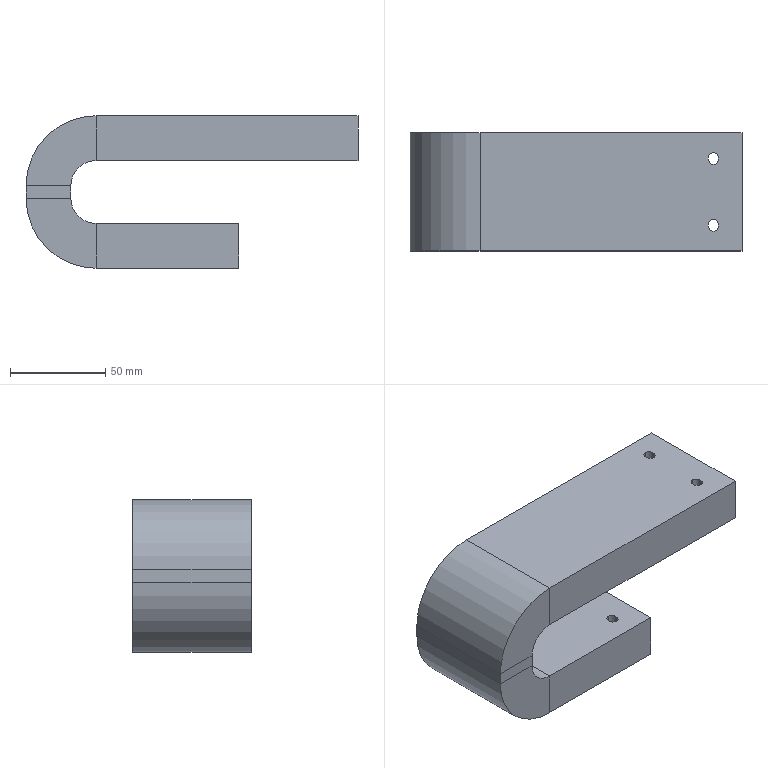Part | SolidWorks | features HoleWzd 2, Sweep 1 | 1 solid | 42 faces | box 174.25 x 62 x 80 mm | volume 431030 mm3 | plane 26 | cylinder 16 | commonest cylinder face diameters 5.2 x12 26.5 x2 73.5 x2
STEP:
#1=CARTESIAN_POINT('',(-15.,-14.4,11.75));
#2=VERTEX_POINT('',#1);
#3=CARTESIAN_POINT('',(-12.4,-17.,11.75));
#4=VERTEX_POINT('',#3);
#5=CARTESIAN_POINT('',(-15.,-17.,11.75));
#6=DIRECTION('',(0.,0.,-1.));
#7=DIRECTION('',(-1.,0.,0.));
#8=AXIS2_PLACEMENT_3D('',#5,#6,#7);
#9=CIRCLE('',#8,2.6);
#10=EDGE_CURVE('',#2,#4,#9,.T.);
#11=ORIENTED_EDGE('',*,*,#10,.F.);
#12=CARTESIAN_POINT('',(-15.,-14.4,-11.75));
#13=VERTEX_POINT('',#12);
#14=CARTESIAN_POINT('',(-15.,-14.4,-11.75));
#15=DIRECTION('',(0.,0.,-1.));
#16=VECTOR('',#15,1000.);
#17=LINE('',#14,#16);
#18=EDGE_CURVE('',#2,#13,#17,.T.);
#19=ORIENTED_EDGE('',*,*,#18,.T.);
#20=CARTESIAN_POINT('',(-12.4,-17.,-11.75));
#21=VERTEX_POINT('',#20);
#22=CARTESIAN_POINT('',(-15.,-17.,-11.75));
#23=DIRECTION('',(0.,0.,-1.));
#24=DIRECTION('',(0.,1.,0.));
#25=AXIS2_PLACEMENT_3D('',#22,#23,#24);
#26=CIRCLE('',#25,2.6);
#27=EDGE_CURVE('',#13,#21,#26,.T.);
#28=ORIENTED_EDGE('',*,*,#27,.T.);
#29=CARTESIAN_POINT('',(-12.4,-17.,23.25));
#30=DIRECTION('',(0.,0.,1.));
#31=VECTOR('',#30,1000.);
#32=LINE('',#29,#31);
#33=EDGE_CURVE('',#21,#4,#32,.T.);
#34=ORIENTED_EDGE('',*,*,#33,.T.);
#35=EDGE_LOOP('',(#11,#19,#28,#34));
#36=FACE_OUTER_BOUND('',#35,.T.);
#37=CARTESIAN_POINT('',(-15.,-17.,-11.75));
#38=DIRECTION('',(0.,0.,-1.));
#39=DIRECTION('',(0.,1.,0.));
#40=AXIS2_PLACEMENT_3D('',#37,#38,#39);
#41=CYLINDRICAL_SURFACE('',#40,2.6);
#42=ADVANCED_FACE('',(#36),#41,.F.);
#43=CARTESIAN_POINT('',(-15.,20.6,11.75));
#44=VERTEX_POINT('',#43);
#45=CARTESIAN_POINT('',(-12.4,18.,11.75));
#46=VERTEX_POINT('',#45);
#47=CARTESIAN_POINT('',(-15.,18.,11.75));
#48=DIRECTION('',(0.,0.,-1.));
#49=DIRECTION('',(-1.,0.,0.));
#50=AXIS2_PLACEMENT_3D('',#47,#48,#49);
#51=CIRCLE('',#50,2.6);
#52=EDGE_CURVE('',#44,#46,#51,.T.);
#53=ORIENTED_EDGE('',*,*,#52,.F.);
#54=CARTESIAN_POINT('',(-15.,20.6,-11.75));
#55=VERTEX_POINT('',#54);
#56=CARTESIAN_POINT('',(-15.,20.6,-11.75));
#57=DIRECTION('',(0.,0.,-1.));
#58=VECTOR('',#57,1000.);
#59=LINE('',#56,#58);
#60=EDGE_CURVE('',#44,#55,#59,.T.);
#61=ORIENTED_EDGE('',*,*,#60,.T.);
#62=CARTESIAN_POINT('',(-12.4,18.,-11.75));
#63=VERTEX_POINT('',#62);
#64=CARTESIAN_POINT('',(-15.,18.,-11.75));
#65=DIRECTION('',(0.,0.,-1.));
#66=DIRECTION('',(0.,1.,0.));
#67=AXIS2_PLACEMENT_3D('',#64,#65,#66);
#68=CIRCLE('',#67,2.6);
#69=EDGE_CURVE('',#55,#63,#68,.T.);
#70=ORIENTED_EDGE('',*,*,#69,.T.);
#71=CARTESIAN_POINT('',(-12.4,18.,23.25));
#72=DIRECTION('',(0.,0.,1.));
#73=VECTOR('',#72,1000.);
#74=LINE('',#71,#73);
#75=EDGE_CURVE('',#63,#46,#74,.T.);
#76=ORIENTED_EDGE('',*,*,#75,.T.);
#77=EDGE_LOOP('',(#53,#61,#70,#76));
#78=FACE_OUTER_BOUND('',#77,.T.);
#79=CARTESIAN_POINT('',(-15.,18.,-11.75));
#80=DIRECTION('',(0.,0.,-1.));
#81=DIRECTION('',(0.,1.,0.));
#82=AXIS2_PLACEMENT_3D('',#79,#80,#81);
#83=CYLINDRICAL_SURFACE('',#82,2.6);
#84=ADVANCED_FACE('',(#78),#83,.F.);
#85=CARTESIAN_POINT('',(47.5,-14.4,68.25));
#86=VERTEX_POINT('',#85);
#87=CARTESIAN_POINT('',(50.1,-17.,68.25));
#88=VERTEX_POINT('',#87);
#89=CARTESIAN_POINT('',(47.5,-17.,68.25));
#90=DIRECTION('',(0.,0.,-1.));
#91=DIRECTION('',(0.,1.,0.));
#92=AXIS2_PLACEMENT_3D('',#89,#90,#91);
#93=CIRCLE('',#92,2.6);
#94=EDGE_CURVE('',#86,#88,#93,.T.);
#95=ORIENTED_EDGE('',*,*,#94,.F.);
#96=CARTESIAN_POINT('',(47.5,-14.4,44.75));
#97=VERTEX_POINT('',#96);
#98=CARTESIAN_POINT('',(47.5,-14.4,44.75));
#99=DIRECTION('',(0.,0.,-1.));
#100=VECTOR('',#99,1000.);
#101=LINE('',#98,#100);
#102=EDGE_CURVE('',#86,#97,#101,.T.);
#103=ORIENTED_EDGE('',*,*,#102,.T.);
#104=CARTESIAN_POINT('',(50.1,-17.,44.75));
#105=VERTEX_POINT('',#104);
#106=CARTESIAN_POINT('',(47.5,-17.,44.75));
#107=DIRECTION('',(0.,0.,-1.));
#108=DIRECTION('',(0.,1.,0.));
#109=AXIS2_PLACEMENT_3D('',#106,#107,#108);
#110=CIRCLE('',#109,2.6);
#111=EDGE_CURVE('',#97,#105,#110,.T.);
#112=ORIENTED_EDGE('',*,*,#111,.T.);
#113=CARTESIAN_POINT('',(50.1,-17.,68.25));
#114=DIRECTION('',(0.,0.,1.));
#115=VECTOR('',#114,1000.);
#116=LINE('',#113,#115);
#117=EDGE_CURVE('',#105,#88,#116,.T.);
#118=ORIENTED_EDGE('',*,*,#117,.T.);
#119=EDGE_LOOP('',(#95,#103,#112,#118));
#120=FACE_OUTER_BOUND('',#119,.T.);
#121=CARTESIAN_POINT('',(47.5,-17.,44.75));
#122=DIRECTION('',(0.,0.,-1.));
#123=DIRECTION('',(0.,1.,0.));
#124=AXIS2_PLACEMENT_3D('',#121,#122,#123);
#125=CYLINDRICAL_SURFACE('',#124,2.6);
#126=ADVANCED_FACE('',(#120),#125,.F.);
#127=CARTESIAN_POINT('',(47.5,20.6,68.25));
#128=VERTEX_POINT('',#127);
#129=CARTESIAN_POINT('',(50.1,18.,68.25));
#130=VERTEX_POINT('',#129);
#131=CARTESIAN_POINT('',(47.5,18.,68.25));
#132=DIRECTION('',(0.,0.,-1.));
#133=DIRECTION('',(0.,1.,0.));
#134=AXIS2_PLACEMENT_3D('',#131,#132,#133);
#135=CIRCLE('',#134,2.6);
#136=EDGE_CURVE('',#128,#130,#135,.T.);
#137=ORIENTED_EDGE('',*,*,#136,.F.);
#138=CARTESIAN_POINT('',(47.5,20.6,44.75));
#139=VERTEX_POINT('',#138);
#140=CARTESIAN_POINT('',(47.5,20.6,44.75));
#141=DIRECTION('',(0.,0.,-1.));
#142=VECTOR('',#141,1000.);
#143=LINE('',#140,#142);
#144=EDGE_CURVE('',#128,#139,#143,.T.);
#145=ORIENTED_EDGE('',*,*,#144,.T.);
#146=CARTESIAN_POINT('',(50.1,18.,44.75));
#147=VERTEX_POINT('',#146);
#148=CARTESIAN_POINT('',(47.5,18.,44.75));
#149=DIRECTION('',(0.,0.,-1.));
#150=DIRECTION('',(0.,1.,0.));
#151=AXIS2_PLACEMENT_3D('',#148,#149,#150);
#152=CIRCLE('',#151,2.6);
#153=EDGE_CURVE('',#139,#147,#152,.T.);
#154=ORIENTED_EDGE('',*,*,#153,.T.);
#155=CARTESIAN_POINT('',(50.1,18.,68.25));
#156=DIRECTION('',(0.,0.,1.));
#157=VECTOR('',#156,1000.);
#158=LINE('',#155,#157);
#159=EDGE_CURVE('',#147,#130,#158,.T.);
#160=ORIENTED_EDGE('',*,*,#159,.T.);
#161=EDGE_LOOP('',(#137,#145,#154,#160));
#162=FACE_OUTER_BOUND('',#161,.T.);
#163=CARTESIAN_POINT('',(47.5,18.,44.75));
#164=DIRECTION('',(0.,0.,-1.));
#165=DIRECTION('',(0.,1.,0.));
#166=AXIS2_PLACEMENT_3D('',#163,#164,#165);
#167=CYLINDRICAL_SURFACE('',#166,2.6);
#168=ADVANCED_FACE('',(#162),#167,.F.);
#169=CARTESIAN_POINT('',(62.5,31.,68.25));
#170=VERTEX_POINT('',#169);
#171=CARTESIAN_POINT('',(62.5,31.,44.75));
#172=VERTEX_POINT('',#171);
#173=CARTESIAN_POINT('',(62.5,31.,68.25));
#174=DIRECTION('',(0.,0.,-1.));
#175=VECTOR('',#174,1000.);
#176=LINE('',#173,#175);
#177=EDGE_CURVE('',#170,#172,#176,.T.);
#178=ORIENTED_EDGE('',*,*,#177,.T.);
#179=CARTESIAN_POINT('',(-75.,31.,44.75));
#180=VERTEX_POINT('',#179);
#181=CARTESIAN_POINT('',(-75.,31.,44.75));
#182=DIRECTION('',(1.,0.,0.));
#183=VECTOR('',#182,1000.);
#184=LINE('',#181,#183);
#185=EDGE_CURVE('',#180,#172,#184,.T.);
#186=ORIENTED_EDGE('',*,*,#185,.F.);
#187=CARTESIAN_POINT('',(-75.,31.,68.25));
#188=VERTEX_POINT('',#187);
#189=CARTESIAN_POINT('',(-75.,31.,68.25));
#190=DIRECTION('',(0.,0.,-1.));
#191=VECTOR('',#190,1000.);
#192=LINE('',#189,#191);
#193=EDGE_CURVE('',#188,#180,#192,.T.);
#194=ORIENTED_EDGE('',*,*,#193,.F.);
#195=CARTESIAN_POINT('',(-75.,31.,68.25));
#196=DIRECTION('',(1.,0.,0.));
#197=VECTOR('',#196,1000.);
#198=LINE('',#195,#197);
#199=EDGE_CURVE('',#188,#170,#198,.T.);
#200=ORIENTED_EDGE('',*,*,#199,.T.);
#201=EDGE_LOOP('',(#178,#186,#194,#200));
#202=FACE_OUTER_BOUND('',#201,.T.);
#203=CARTESIAN_POINT('',(-75.,31.,68.25));
#204=DIRECTION('',(0.,-1.,0.));
#205=DIRECTION('',(0.,0.,-1.));
#206=AXIS2_PLACEMENT_3D('',#203,#204,#205);
#207=PLANE('',#206);
#208=ADVANCED_FACE('',(#202),#207,.F.);
#209=CARTESIAN_POINT('',(50.1,-18.,68.25));
#210=VERTEX_POINT('',#209);
#211=CARTESIAN_POINT('',(44.9,-18.,68.25));
#212=VERTEX_POINT('',#211);
#213=CARTESIAN_POINT('',(47.5,-18.,68.25));
#214=DIRECTION('',(0.,0.,-1.));
#215=DIRECTION('',(0.,1.,0.));
#216=AXIS2_PLACEMENT_3D('',#213,#214,#215);
#217=CIRCLE('',#216,2.6);
#218=EDGE_CURVE('',#210,#212,#217,.T.);
#219=ORIENTED_EDGE('',*,*,#218,.T.);
#220=CARTESIAN_POINT('',(44.9,-17.,68.25));
#221=VERTEX_POINT('',#220);
#222=CARTESIAN_POINT('',(44.9,-18.,68.25));
#223=DIRECTION('',(0.,1.,0.));
#224=VECTOR('',#223,1000.);
#225=LINE('',#222,#224);
#226=EDGE_CURVE('',#212,#221,#225,.T.);
#227=ORIENTED_EDGE('',*,*,#226,.T.);
#228=CARTESIAN_POINT('',(47.5,-17.,68.25));
#229=DIRECTION('',(0.,0.,-1.));
#230=DIRECTION('',(0.,1.,0.));
#231=AXIS2_PLACEMENT_3D('',#228,#229,#230);
#232=CIRCLE('',#231,2.6);
#233=EDGE_CURVE('',#221,#86,#232,.T.);
#234=ORIENTED_EDGE('',*,*,#233,.T.);
#235=ORIENTED_EDGE('',*,*,#94,.T.);
#236=CARTESIAN_POINT('',(50.1,-18.,68.25));
#237=DIRECTION('',(0.,1.,0.));
#238=VECTOR('',#237,1000.);
#239=LINE('',#236,#238);
#240=EDGE_CURVE('',#210,#88,#239,.T.);
#241=ORIENTED_EDGE('',*,*,#240,.F.);
#242=EDGE_LOOP('',(#219,#227,#234,#235,#241));
#243=FACE_BOUND('',#242,.T.);
#244=CARTESIAN_POINT('',(50.1,17.,68.25));
#245=VERTEX_POINT('',#244);
#246=CARTESIAN_POINT('',(44.9,17.,68.25));
#247=VERTEX_POINT('',#246);
#248=CARTESIAN_POINT('',(47.5,17.,68.25));
#249=DIRECTION('',(0.,0.,-1.));
#250=DIRECTION('',(0.,1.,0.));
#251=AXIS2_PLACEMENT_3D('',#248,#249,#250);
#252=CIRCLE('',#251,2.6);
#253=EDGE_CURVE('',#245,#247,#252,.T.);
#254=ORIENTED_EDGE('',*,*,#253,.T.);
#255=CARTESIAN_POINT('',(44.9,18.,68.25));
#256=VERTEX_POINT('',#255);
#257=CARTESIAN_POINT('',(44.9,17.,68.25));
#258=DIRECTION('',(0.,1.,0.));
#259=VECTOR('',#258,1000.);
#260=LINE('',#257,#259);
#261=EDGE_CURVE('',#247,#256,#260,.T.);
#262=ORIENTED_EDGE('',*,*,#261,.T.);
#263=CARTESIAN_POINT('',(47.5,18.,68.25));
#264=DIRECTION('',(0.,0.,-1.));
#265=DIRECTION('',(0.,1.,0.));
#266=AXIS2_PLACEMENT_3D('',#263,#264,#265);
#267=CIRCLE('',#266,2.6);
#268=EDGE_CURVE('',#256,#128,#267,.T.);
#269=ORIENTED_EDGE('',*,*,#268,.T.);
#270=ORIENTED_EDGE('',*,*,#136,.T.);
#271=CARTESIAN_POINT('',(50.1,17.,68.25));
#272=DIRECTION('',(0.,1.,0.));
#273=VECTOR('',#272,1000.);
#274=LINE('',#271,#273);
#275=EDGE_CURVE('',#245,#130,#274,.T.);
#276=ORIENTED_EDGE('',*,*,#275,.F.);
#277=EDGE_LOOP('',(#254,#262,#269,#270,#276));
#278=FACE_BOUND('',#277,.T.);
#279=ORIENTED_EDGE('',*,*,#199,.F.);
#280=CARTESIAN_POINT('',(-75.,-31.,68.25));
#281=VERTEX_POINT('',#280);
#282=CARTESIAN_POINT('',(-75.,31.,68.25));
#283=DIRECTION('',(0.,1.,0.));
#284=VECTOR('',#283,1000.);
#285=LINE('',#282,#284);
#286=EDGE_CURVE('',#281,#188,#285,.T.);
#287=ORIENTED_EDGE('',*,*,#286,.F.);
#288=CARTESIAN_POINT('',(62.5,-31.,68.25));
#289=VERTEX_POINT('',#288);
#290=CARTESIAN_POINT('',(-75.,-31.,68.25));
#291=DIRECTION('',(1.,0.,0.));
#292=VECTOR('',#291,1000.);
#293=LINE('',#290,#292);
#294=EDGE_CURVE('',#281,#289,#293,.T.);
#295=ORIENTED_EDGE('',*,*,#294,.T.);
#296=CARTESIAN_POINT('',(62.5,31.,68.25));
#297=DIRECTION('',(0.,1.,0.));
#298=VECTOR('',#297,1000.);
#299=LINE('',#296,#298);
#300=EDGE_CURVE('',#289,#170,#299,.T.);
#301=ORIENTED_EDGE('',*,*,#300,.T.);
#302=EDGE_LOOP('',(#279,#287,#295,#301));
#303=FACE_OUTER_BOUND('',#302,.T.);
#304=CARTESIAN_POINT('',(-75.,31.,68.25));
#305=DIRECTION('',(0.,0.,-1.));
#306=DIRECTION('',(0.,1.,0.));
#307=AXIS2_PLACEMENT_3D('',#304,#305,#306);
#308=PLANE('',#307);
#309=ADVANCED_FACE('',(#243,#278,#303),#308,.F.);
#310=ORIENTED_EDGE('',*,*,#294,.F.);
#311=CARTESIAN_POINT('',(-75.,-31.,44.75));
#312=VERTEX_POINT('',#311);
#313=CARTESIAN_POINT('',(-75.,-31.,68.25));
#314=DIRECTION('',(0.,0.,1.));
#315=VECTOR('',#314,1000.);
#316=LINE('',#313,#315);
#317=EDGE_CURVE('',#312,#281,#316,.T.);
#318=ORIENTED_EDGE('',*,*,#317,.F.);
#319=CARTESIAN_POINT('',(62.5,-31.,44.75));
#320=VERTEX_POINT('',#319);
#321=CARTESIAN_POINT('',(-75.,-31.,44.75));
#322=DIRECTION('',(1.,0.,0.));
#323=VECTOR('',#322,1000.);
#324=LINE('',#321,#323);
#325=EDGE_CURVE('',#312,#320,#324,.T.);
#326=ORIENTED_EDGE('',*,*,#325,.T.);
#327=CARTESIAN_POINT('',(62.5,-31.,68.25));
#328=DIRECTION('',(0.,0.,1.));
#329=VECTOR('',#328,1000.);
#330=LINE('',#327,#329);
#331=EDGE_CURVE('',#320,#289,#330,.T.);
#332=ORIENTED_EDGE('',*,*,#331,.T.);
#333=EDGE_LOOP('',(#310,#318,#326,#332));
#334=FACE_OUTER_BOUND('',#333,.T.);
#335=CARTESIAN_POINT('',(-75.,-31.,68.25));
#336=DIRECTION('',(0.,1.,0.));
#337=DIRECTION('',(0.,0.,1.));
#338=AXIS2_PLACEMENT_3D('',#335,#336,#337);
#339=PLANE('',#338);
#340=ADVANCED_FACE('',(#334),#339,.F.);
#341=CARTESIAN_POINT('',(50.1,-18.,44.75));
#342=VERTEX_POINT('',#341);
#343=CARTESIAN_POINT('',(50.1,-18.,44.75));
#344=DIRECTION('',(0.,1.,0.));
#345=VECTOR('',#344,1000.);
#346=LINE('',#343,#345);
#347=EDGE_CURVE('',#342,#105,#346,.T.);
#348=ORIENTED_EDGE('',*,*,#347,.T.);
#349=ORIENTED_EDGE('',*,*,#111,.F.);
#350=CARTESIAN_POINT('',(44.9,-17.,44.75));
#351=VERTEX_POINT('',#350);
#352=CARTESIAN_POINT('',(47.5,-17.,44.75));
#353=DIRECTION('',(0.,0.,-1.));
#354=DIRECTION('',(0.,1.,0.));
#355=AXIS2_PLACEMENT_3D('',#352,#353,#354);
#356=CIRCLE('',#355,2.6);
#357=EDGE_CURVE('',#351,#97,#356,.T.);
#358=ORIENTED_EDGE('',*,*,#357,.F.);
#359=CARTESIAN_POINT('',(44.9,-18.,44.75));
#360=VERTEX_POINT('',#359);
#361=CARTESIAN_POINT('',(44.9,-18.,44.75));
#362=DIRECTION('',(0.,1.,0.));
#363=VECTOR('',#362,1000.);
#364=LINE('',#361,#363);
#365=EDGE_CURVE('',#360,#351,#364,.T.);
#366=ORIENTED_EDGE('',*,*,#365,.F.);
#367=CARTESIAN_POINT('',(47.5,-18.,44.75));
#368=DIRECTION('',(0.,0.,-1.));
#369=DIRECTION('',(0.,1.,0.));
#370=AXIS2_PLACEMENT_3D('',#367,#368,#369);
#371=CIRCLE('',#370,2.6);
#372=EDGE_CURVE('',#342,#360,#371,.T.);
#373=ORIENTED_EDGE('',*,*,#372,.F.);
#374=EDGE_LOOP('',(#348,#349,#358,#366,#373));
#375=FACE_BOUND('',#374,.T.);
#376=CARTESIAN_POINT('',(44.9,18.,44.75));
#377=VERTEX_POINT('',#376);
#378=CARTESIAN_POINT('',(47.5,18.,44.75));
#379=DIRECTION('',(0.,0.,-1.));
#380=DIRECTION('',(0.,1.,0.));
#381=AXIS2_PLACEMENT_3D('',#378,#379,#380);
#382=CIRCLE('',#381,2.6);
#383=EDGE_CURVE('',#377,#139,#382,.T.);
#384=ORIENTED_EDGE('',*,*,#383,.F.);
#385=CARTESIAN_POINT('',(44.9,17.,44.75));
#386=VERTEX_POINT('',#385);
#387=CARTESIAN_POINT('',(44.9,17.,44.75));
#388=DIRECTION('',(0.,1.,0.));
#389=VECTOR('',#388,1000.);
#390=LINE('',#387,#389);
#391=EDGE_CURVE('',#386,#377,#390,.T.);
#392=ORIENTED_EDGE('',*,*,#391,.F.);
#393=CARTESIAN_POINT('',(50.1,17.,44.75));
#394=VERTEX_POINT('',#393);
#395=CARTESIAN_POINT('',(47.5,17.,44.75));
#396=DIRECTION('',(0.,0.,-1.));
#397=DIRECTION('',(0.,1.,0.));
#398=AXIS2_PLACEMENT_3D('',#395,#396,#397);
#399=CIRCLE('',#398,2.6);
#400=EDGE_CURVE('',#394,#386,#399,.T.);
#401=ORIENTED_EDGE('',*,*,#400,.F.);
#402=CARTESIAN_POINT('',(50.1,17.,44.75));
#403=DIRECTION('',(0.,1.,0.));
#404=VECTOR('',#403,1000.);
#405=LINE('',#402,#404);
#406=EDGE_CURVE('',#394,#147,#405,.T.);
#407=ORIENTED_EDGE('',*,*,#406,.T.);
#408=ORIENTED_EDGE('',*,*,#153,.F.);
#409=EDGE_LOOP('',(#384,#392,#401,#407,#408));
#410=FACE_BOUND('',#409,.T.);
#411=ORIENTED_EDGE('',*,*,#325,.F.);
#412=CARTESIAN_POINT('',(-75.,31.,44.75));
#413=DIRECTION('',(0.,-1.,0.));
#414=VECTOR('',#413,1000.);
#415=LINE('',#412,#414);
#416=EDGE_CURVE('',#180,#312,#415,.T.);
#417=ORIENTED_EDGE('',*,*,#416,.F.);
#418=ORIENTED_EDGE('',*,*,#185,.T.);
#419=CARTESIAN_POINT('',(62.5,31.,44.75));
#420=DIRECTION('',(0.,-1.,0.));
#421=VECTOR('',#420,1000.);
#422=LINE('',#419,#421);
#423=EDGE_CURVE('',#172,#320,#422,.T.);
#424=ORIENTED_EDGE('',*,*,#423,.T.);
#425=EDGE_LOOP('',(#411,#417,#418,#424));
#426=FACE_OUTER_BOUND('',#425,.T.);
#427=CARTESIAN_POINT('',(-75.,31.,44.75));
#428=DIRECTION('',(0.,0.,1.));
#429=DIRECTION('',(0.,-1.,0.));
#430=AXIS2_PLACEMENT_3D('',#427,#428,#429);
#431=PLANE('',#430);
#432=ADVANCED_FACE('',(#375,#410,#426),#431,.F.);
#433=ORIENTED_EDGE('',*,*,#193,.T.);
#434=CARTESIAN_POINT('',(-88.25,31.,31.5));
#435=VERTEX_POINT('',#434);
#436=CARTESIAN_POINT('',(-75.,31.,31.5));
#437=DIRECTION('',(0.,1.,0.));
#438=DIRECTION('',(-1.,0.,0.));
#439=AXIS2_PLACEMENT_3D('',#436,#437,#438);
#440=CIRCLE('',#439,13.25);
#441=EDGE_CURVE('',#435,#180,#440,.T.);
#442=ORIENTED_EDGE('',*,*,#441,.F.);
#443=CARTESIAN_POINT('',(-111.75,31.,31.5));
#444=VERTEX_POINT('',#443);
#445=CARTESIAN_POINT('',(-111.75,31.,31.5));
#446=DIRECTION('',(1.,0.,0.));
#447=VECTOR('',#446,1000.);
#448=LINE('',#445,#447);
#449=EDGE_CURVE('',#444,#435,#448,.T.);
#450=ORIENTED_EDGE('',*,*,#449,.F.);
#451=CARTESIAN_POINT('',(-75.,31.,31.5));
#452=DIRECTION('',(0.,1.,0.));
#453=DIRECTION('',(-1.,0.,0.));
#454=AXIS2_PLACEMENT_3D('',#451,#452,#453);
#455=CIRCLE('',#454,36.75);
#456=EDGE_CURVE('',#444,#188,#455,.T.);
#457=ORIENTED_EDGE('',*,*,#456,.T.);
#458=EDGE_LOOP('',(#433,#442,#450,#457));
#459=FACE_OUTER_BOUND('',#458,.T.);
#460=CARTESIAN_POINT('',(-111.75,31.,31.5));
#461=DIRECTION('',(0.,-1.,0.));
#462=DIRECTION('',(0.,0.,-1.));
#463=AXIS2_PLACEMENT_3D('',#460,#461,#462);
#464=PLANE('',#463);
#465=ADVANCED_FACE('',(#459),#464,.F.);
#466=ORIENTED_EDGE('',*,*,#456,.F.);
#467=CARTESIAN_POINT('',(-111.75,-31.,31.5));
#468=VERTEX_POINT('',#467);
#469=CARTESIAN_POINT('',(-111.75,31.,31.5));
#470=DIRECTION('',(0.,1.,0.));
#471=VECTOR('',#470,1000.);
#472=LINE('',#469,#471);
#473=EDGE_CURVE('',#468,#444,#472,.T.);
#474=ORIENTED_EDGE('',*,*,#473,.F.);
#475=CARTESIAN_POINT('',(-75.,-31.,31.5));
#476=DIRECTION('',(0.,1.,0.));
#477=DIRECTION('',(-1.,0.,0.));
#478=AXIS2_PLACEMENT_3D('',#475,#476,#477);
#479=CIRCLE('',#478,36.75);
#480=EDGE_CURVE('',#468,#281,#479,.T.);
#481=ORIENTED_EDGE('',*,*,#480,.T.);
#482=ORIENTED_EDGE('',*,*,#286,.T.);
#483=EDGE_LOOP('',(#466,#474,#481,#482));
#484=FACE_OUTER_BOUND('',#483,.T.);
#485=CARTESIAN_POINT('',(-75.,0.,31.5));
#486=DIRECTION('',(0.,1.,0.));
#487=DIRECTION('',(0.,0.,1.));
#488=AXIS2_PLACEMENT_3D('',#485,#486,#487);
#489=CYLINDRICAL_SURFACE('',#488,36.75);
#490=ADVANCED_FACE('',(#484),#489,.T.);
#491=ORIENTED_EDGE('',*,*,#480,.F.);
#492=CARTESIAN_POINT('',(-88.25,-31.,31.5));
#493=VERTEX_POINT('',#492);
#494=CARTESIAN_POINT('',(-111.75,-31.,31.5));
#495=DIRECTION('',(-1.,0.,0.));
#496=VECTOR('',#495,1000.);
#497=LINE('',#494,#496);
#498=EDGE_CURVE('',#493,#468,#497,.T.);
#499=ORIENTED_EDGE('',*,*,#498,.F.);
#500=CARTESIAN_POINT('',(-75.,-31.,31.5));
#501=DIRECTION('',(0.,1.,0.));
#502=DIRECTION('',(-1.,0.,0.));
#503=AXIS2_PLACEMENT_3D('',#500,#501,#502);
#504=CIRCLE('',#503,13.25);
#505=EDGE_CURVE('',#493,#312,#504,.T.);
#506=ORIENTED_EDGE('',*,*,#505,.T.);
#507=ORIENTED_EDGE('',*,*,#317,.T.);
#508=EDGE_LOOP('',(#491,#499,#506,#507));
#509=FACE_OUTER_BOUND('',#508,.T.);
#510=CARTESIAN_POINT('',(-111.75,-31.,31.5));
#511=DIRECTION('',(0.,1.,0.));
#512=DIRECTION('',(0.,0.,1.));
#513=AXIS2_PLACEMENT_3D('',#510,#511,#512);
#514=PLANE('',#513);
#515=ADVANCED_FACE('',(#509),#514,.F.);
#516=ORIENTED_EDGE('',*,*,#505,.F.);
#517=CARTESIAN_POINT('',(-88.25,31.,31.5));
#518=DIRECTION('',(0.,-1.,0.));
#519=VECTOR('',#518,1000.);
#520=LINE('',#517,#519);
#521=EDGE_CURVE('',#435,#493,#520,.T.);
#522=ORIENTED_EDGE('',*,*,#521,.F.);
#523=ORIENTED_EDGE('',*,*,#441,.T.);
#524=ORIENTED_EDGE('',*,*,#416,.T.);
#525=EDGE_LOOP('',(#516,#522,#523,#524));
#526=FACE_OUTER_BOUND('',#525,.T.);
#527=CARTESIAN_POINT('',(-75.,0.,31.5));
#528=DIRECTION('',(0.,1.,0.));
#529=DIRECTION('',(0.,0.,1.));
#530=AXIS2_PLACEMENT_3D('',#527,#528,#529);
#531=CYLINDRICAL_SURFACE('',#530,13.25);
#532=ADVANCED_FACE('',(#526),#531,.F.);
#533=ORIENTED_EDGE('',*,*,#449,.T.);
#534=CARTESIAN_POINT('',(-88.25,31.,25.));
#535=VERTEX_POINT('',#534);
#536=CARTESIAN_POINT('',(-88.25,31.,25.));
#537=DIRECTION('',(0.,0.,1.));
#538=VECTOR('',#537,1000.);
#539=LINE('',#536,#538);
#540=EDGE_CURVE('',#535,#435,#539,.T.);
#541=ORIENTED_EDGE('',*,*,#540,.F.);
#542=CARTESIAN_POINT('',(-111.75,31.,25.));
#543=VERTEX_POINT('',#542);
#544=CARTESIAN_POINT('',(-111.75,31.,25.));
#545=DIRECTION('',(1.,0.,0.));
#546=VECTOR('',#545,1000.);
#547=LINE('',#544,#546);
#548=EDGE_CURVE('',#543,#535,#547,.T.);
#549=ORIENTED_EDGE('',*,*,#548,.F.);
#550=CARTESIAN_POINT('',(-111.75,31.,25.));
#551=DIRECTION('',(0.,0.,1.));
#552=VECTOR('',#551,1000.);
#553=LINE('',#550,#552);
#554=EDGE_CURVE('',#543,#444,#553,.T.);
#555=ORIENTED_EDGE('',*,*,#554,.T.);
#556=EDGE_LOOP('',(#533,#541,#549,#555));
#557=FACE_OUTER_BOUND('',#556,.T.);
#558=CARTESIAN_POINT('',(-111.75,31.,25.));
#559=DIRECTION('',(0.,-1.,0.));
#560=DIRECTION('',(0.,0.,-1.));
#561=AXIS2_PLACEMENT_3D('',#558,#559,#560);
#562=PLANE('',#561);
#563=ADVANCED_FACE('',(#557),#562,.F.);
#564=ORIENTED_EDGE('',*,*,#554,.F.);
#565=CARTESIAN_POINT('',(-111.75,-31.,25.));
#566=VERTEX_POINT('',#565);
#567=CARTESIAN_POINT('',(-111.75,31.,25.));
#568=DIRECTION('',(0.,1.,0.));
#569=VECTOR('',#568,1000.);
#570=LINE('',#567,#569);
#571=EDGE_CURVE('',#566,#543,#570,.T.);
#572=ORIENTED_EDGE('',*,*,#571,.F.);
#573=CARTESIAN_POINT('',(-111.75,-31.,25.));
#574=DIRECTION('',(0.,0.,1.));
#575=VECTOR('',#574,1000.);
#576=LINE('',#573,#575);
#577=EDGE_CURVE('',#566,#468,#576,.T.);
#578=ORIENTED_EDGE('',*,*,#577,.T.);
#579=ORIENTED_EDGE('',*,*,#473,.T.);
#580=EDGE_LOOP('',(#564,#572,#578,#579));
#581=FACE_OUTER_BOUND('',#580,.T.);
#582=CARTESIAN_POINT('',(-111.75,31.,25.));
#583=DIRECTION('',(1.,0.,0.));
#584=DIRECTION('',(0.,1.,0.));
#585=AXIS2_PLACEMENT_3D('',#582,#583,#584);
#586=PLANE('',#585);
#587=ADVANCED_FACE('',(#581),#586,.F.);
#588=ORIENTED_EDGE('',*,*,#577,.F.);
#589=CARTESIAN_POINT('',(-88.25,-31.,25.));
#590=VERTEX_POINT('',#589);
#591=CARTESIAN_POINT('',(-111.75,-31.,25.));
#592=DIRECTION('',(-1.,0.,0.));
#593=VECTOR('',#592,1000.);
#594=LINE('',#591,#593);
#595=EDGE_CURVE('',#590,#566,#594,.T.);
#596=ORIENTED_EDGE('',*,*,#595,.F.);
#597=CARTESIAN_POINT('',(-88.25,-31.,25.));
#598=DIRECTION('',(0.,0.,1.));
#599=VECTOR('',#598,1000.);
#600=LINE('',#597,#599);
#601=EDGE_CURVE('',#590,#493,#600,.T.);
#602=ORIENTED_EDGE('',*,*,#601,.T.);
#603=ORIENTED_EDGE('',*,*,#498,.T.);
#604=EDGE_LOOP('',(#588,#596,#602,#603));
#605=FACE_OUTER_BOUND('',#604,.T.);
#606=CARTESIAN_POINT('',(-111.75,-31.,25.));
#607=DIRECTION('',(0.,1.,0.));
#608=DIRECTION('',(0.,0.,1.));
#609=AXIS2_PLACEMENT_3D('',#606,#607,#608);
#610=PLANE('',#609);
#611=ADVANCED_FACE('',(#605),#610,.F.);
#612=ORIENTED_EDGE('',*,*,#601,.F.);
#613=CARTESIAN_POINT('',(-88.25,31.,25.));
#614=DIRECTION('',(0.,-1.,0.));
#615=VECTOR('',#614,1000.);
#616=LINE('',#613,#615);
#617=EDGE_CURVE('',#535,#590,#616,.T.);
#618=ORIENTED_EDGE('',*,*,#617,.F.);
#619=ORIENTED_EDGE('',*,*,#540,.T.);
#620=ORIENTED_EDGE('',*,*,#521,.T.);
#621=EDGE_LOOP('',(#612,#618,#619,#620));
#622=FACE_OUTER_BOUND('',#621,.T.);
#623=CARTESIAN_POINT('',(-88.25,31.,25.));
#624=DIRECTION('',(-1.,0.,0.));
#625=DIRECTION('',(0.,-1.,0.));
#626=AXIS2_PLACEMENT_3D('',#623,#624,#625);
#627=PLANE('',#626);
#628=ADVANCED_FACE('',(#622),#627,.F.);
#629=ORIENTED_EDGE('',*,*,#548,.T.);
#630=CARTESIAN_POINT('',(-75.,31.,11.75));
#631=VERTEX_POINT('',#630);
#632=CARTESIAN_POINT('',(-75.,31.,25.));
#633=DIRECTION('',(0.,1.,0.));
#634=DIRECTION('',(0.,0.,-1.));
#635=AXIS2_PLACEMENT_3D('',#632,#633,#634);
#636=CIRCLE('',#635,13.25);
#637=EDGE_CURVE('',#631,#535,#636,.T.);
#638=ORIENTED_EDGE('',*,*,#637,.F.);
#639=CARTESIAN_POINT('',(-75.,31.,-11.75));
#640=VERTEX_POINT('',#639);
#641=CARTESIAN_POINT('',(-75.,31.,-11.75));
#642=DIRECTION('',(0.,0.,1.));
#643=VECTOR('',#642,1000.);
#644=LINE('',#641,#643);
#645=EDGE_CURVE('',#640,#631,#644,.T.);
#646=ORIENTED_EDGE('',*,*,#645,.F.);
#647=CARTESIAN_POINT('',(-75.,31.,25.));
#648=DIRECTION('',(0.,1.,0.));
#649=DIRECTION('',(0.,0.,-1.));
#650=AXIS2_PLACEMENT_3D('',#647,#648,#649);
#651=CIRCLE('',#650,36.75);
#652=EDGE_CURVE('',#640,#543,#651,.T.);
#653=ORIENTED_EDGE('',*,*,#652,.T.);
#654=EDGE_LOOP('',(#629,#638,#646,#653));
#655=FACE_OUTER_BOUND('',#654,.T.);
#656=CARTESIAN_POINT('',(-75.,31.,-11.75));
#657=DIRECTION('',(0.,-1.,0.));
#658=DIRECTION('',(0.,0.,-1.));
#659=AXIS2_PLACEMENT_3D('',#656,#657,#658);
#660=PLANE('',#659);
#661=ADVANCED_FACE('',(#655),#660,.F.);
#662=ORIENTED_EDGE('',*,*,#652,.F.);
#663=CARTESIAN_POINT('',(-75.,-31.,-11.75));
#664=VERTEX_POINT('',#663);
#665=CARTESIAN_POINT('',(-75.,31.,-11.75));
#666=DIRECTION('',(0.,1.,0.));
#667=VECTOR('',#666,1000.);
#668=LINE('',#665,#667);
#669=EDGE_CURVE('',#664,#640,#668,.T.);
#670=ORIENTED_EDGE('',*,*,#669,.F.);
#671=CARTESIAN_POINT('',(-75.,-31.,25.));
#672=DIRECTION('',(0.,1.,0.));
#673=DIRECTION('',(0.,0.,-1.));
#674=AXIS2_PLACEMENT_3D('',#671,#672,#673);
#675=CIRCLE('',#674,36.75);
#676=EDGE_CURVE('',#664,#566,#675,.T.);
#677=ORIENTED_EDGE('',*,*,#676,.T.);
#678=ORIENTED_EDGE('',*,*,#571,.T.);
#679=EDGE_LOOP('',(#662,#670,#677,#678));
#680=FACE_OUTER_BOUND('',#679,.T.);
#681=CARTESIAN_POINT('',(-75.,0.,25.));
#682=DIRECTION('',(0.,1.,0.));
#683=DIRECTION('',(0.,0.,1.));
#684=AXIS2_PLACEMENT_3D('',#681,#682,#683);
#685=CYLINDRICAL_SURFACE('',#684,36.75);
#686=ADVANCED_FACE('',(#680),#685,.T.);
#687=ORIENTED_EDGE('',*,*,#676,.F.);
#688=CARTESIAN_POINT('',(-75.,-31.,11.75));
#689=VERTEX_POINT('',#688);
#690=CARTESIAN_POINT('',(-75.,-31.,-11.75));
#691=DIRECTION('',(0.,0.,-1.));
#692=VECTOR('',#691,1000.);
#693=LINE('',#690,#692);
#694=EDGE_CURVE('',#689,#664,#693,.T.);
#695=ORIENTED_EDGE('',*,*,#694,.F.);
#696=CARTESIAN_POINT('',(-75.,-31.,25.));
#697=DIRECTION('',(0.,1.,0.));
#698=DIRECTION('',(0.,0.,-1.));
#699=AXIS2_PLACEMENT_3D('',#696,#697,#698);
#700=CIRCLE('',#699,13.25);
#701=EDGE_CURVE('',#689,#590,#700,.T.);
#702=ORIENTED_EDGE('',*,*,#701,.T.);
#703=ORIENTED_EDGE('',*,*,#595,.T.);
#704=EDGE_LOOP('',(#687,#695,#702,#703));
#705=FACE_OUTER_BOUND('',#704,.T.);
#706=CARTESIAN_POINT('',(-75.,-31.,-11.75));
#707=DIRECTION('',(0.,1.,0.));
#708=DIRECTION('',(0.,0.,1.));
#709=AXIS2_PLACEMENT_3D('',#706,#707,#708);
#710=PLANE('',#709);
#711=ADVANCED_FACE('',(#705),#710,.F.);
#712=ORIENTED_EDGE('',*,*,#701,.F.);
#713=CARTESIAN_POINT('',(-75.,31.,11.75));
#714=DIRECTION('',(0.,-1.,0.));
#715=VECTOR('',#714,1000.);
#716=LINE('',#713,#715);
#717=EDGE_CURVE('',#631,#689,#716,.T.);
#718=ORIENTED_EDGE('',*,*,#717,.F.);
#719=ORIENTED_EDGE('',*,*,#637,.T.);
#720=ORIENTED_EDGE('',*,*,#617,.T.);
#721=EDGE_LOOP('',(#712,#718,#719,#720));
#722=FACE_OUTER_BOUND('',#721,.T.);
#723=CARTESIAN_POINT('',(-75.,0.,25.));
#724=DIRECTION('',(0.,1.,0.));
#725=DIRECTION('',(0.,0.,1.));
#726=AXIS2_PLACEMENT_3D('',#723,#724,#725);
#727=CYLINDRICAL_SURFACE('',#726,13.25);
#728=ADVANCED_FACE('',(#722),#727,.F.);
#729=ORIENTED_EDGE('',*,*,#645,.T.);
#730=CARTESIAN_POINT('',(0.,31.,11.75));
#731=VERTEX_POINT('',#730);
#732=CARTESIAN_POINT('',(0.,31.,11.75));
#733=DIRECTION('',(-1.,0.,0.));
#734=VECTOR('',#733,1000.);
#735=LINE('',#732,#734);
#736=EDGE_CURVE('',#731,#631,#735,.T.);
#737=ORIENTED_EDGE('',*,*,#736,.F.);
#738=CARTESIAN_POINT('',(0.,31.,-11.75));
#739=VERTEX_POINT('',#738);
#740=CARTESIAN_POINT('',(0.,31.,-11.75));
#741=DIRECTION('',(0.,0.,1.));
#742=VECTOR('',#741,1000.);
#743=LINE('',#740,#742);
#744=EDGE_CURVE('',#739,#731,#743,.T.);
#745=ORIENTED_EDGE('',*,*,#744,.F.);
#746=CARTESIAN_POINT('',(0.,31.,-11.75));
#747=DIRECTION('',(-1.,0.,0.));
#748=VECTOR('',#747,1000.);
#749=LINE('',#746,#748);
#750=EDGE_CURVE('',#739,#640,#749,.T.);
#751=ORIENTED_EDGE('',*,*,#750,.T.);
#752=EDGE_LOOP('',(#729,#737,#745,#751));
#753=FACE_OUTER_BOUND('',#752,.T.);
#754=CARTESIAN_POINT('',(0.,31.,-11.75));
#755=DIRECTION('',(0.,-1.,0.));
#756=DIRECTION('',(0.,0.,-1.));
#757=AXIS2_PLACEMENT_3D('',#754,#755,#756);
#758=PLANE('',#757);
#759=ADVANCED_FACE('',(#753),#758,.F.);
#760=CARTESIAN_POINT('',(-12.4,-18.,-11.75));
#761=VERTEX_POINT('',#760);
#762=CARTESIAN_POINT('',(-17.6,-18.,-11.75));
#763=VERTEX_POINT('',#762);
#764=CARTESIAN_POINT('',(-15.,-18.,-11.75));
#765=DIRECTION('',(0.,0.,-1.));
#766=DIRECTION('',(0.,1.,0.));
#767=AXIS2_PLACEMENT_3D('',#764,#765,#766);
#768=CIRCLE('',#767,2.6);
#769=EDGE_CURVE('',#761,#763,#768,.T.);
#770=ORIENTED_EDGE('',*,*,#769,.F.);
#771=CARTESIAN_POINT('',(-12.4,-17.,-11.75));
#772=DIRECTION('',(0.,-1.,0.));
#773=VECTOR('',#772,1000.);
#774=LINE('',#771,#773);
#775=EDGE_CURVE('',#21,#761,#774,.T.);
#776=ORIENTED_EDGE('',*,*,#775,.F.);
#777=ORIENTED_EDGE('',*,*,#27,.F.);
#778=CARTESIAN_POINT('',(-17.6,-17.,-11.75));
#779=VERTEX_POINT('',#778);
#780=CARTESIAN_POINT('',(-15.,-17.,-11.75));
#781=DIRECTION('',(0.,0.,-1.));
#782=DIRECTION('',(0.,1.,0.));
#783=AXIS2_PLACEMENT_3D('',#780,#781,#782);
#784=CIRCLE('',#783,2.6);
#785=EDGE_CURVE('',#779,#13,#784,.T.);
#786=ORIENTED_EDGE('',*,*,#785,.F.);
#787=CARTESIAN_POINT('',(-17.6,-17.,-11.75));
#788=DIRECTION('',(0.,-1.,0.));
#789=VECTOR('',#788,1000.);
#790=LINE('',#787,#789);
#791=EDGE_CURVE('',#779,#763,#790,.T.);
#792=ORIENTED_EDGE('',*,*,#791,.T.);
#793=EDGE_LOOP('',(#770,#776,#777,#786,#792));
#794=FACE_BOUND('',#793,.T.);
#795=CARTESIAN_POINT('',(-17.6,18.,-11.75));
#796=VERTEX_POINT('',#795);
#797=CARTESIAN_POINT('',(-15.,18.,-11.75));
#798=DIRECTION('',(0.,0.,-1.));
#799=DIRECTION('',(0.,1.,0.));
#800=AXIS2_PLACEMENT_3D('',#797,#798,#799);
#801=CIRCLE('',#800,2.6);
#802=EDGE_CURVE('',#796,#55,#801,.T.);
#803=ORIENTED_EDGE('',*,*,#802,.F.);
#804=CARTESIAN_POINT('',(-17.6,17.,-11.75));
#805=VERTEX_POINT('',#804);
#806=CARTESIAN_POINT('',(-17.6,18.,-11.75));
#807=DIRECTION('',(0.,-1.,0.));
#808=VECTOR('',#807,1000.);
#809=LINE('',#806,#808);
#810=EDGE_CURVE('',#796,#805,#809,.T.);
#811=ORIENTED_EDGE('',*,*,#810,.T.);
#812=CARTESIAN_POINT('',(-12.4,17.,-11.75));
#813=VERTEX_POINT('',#812);
#814=CARTESIAN_POINT('',(-15.,17.,-11.75));
#815=DIRECTION('',(0.,0.,-1.));
#816=DIRECTION('',(0.,1.,0.));
#817=AXIS2_PLACEMENT_3D('',#814,#815,#816);
#818=CIRCLE('',#817,2.6);
#819=EDGE_CURVE('',#813,#805,#818,.T.);
#820=ORIENTED_EDGE('',*,*,#819,.F.);
#821=CARTESIAN_POINT('',(-12.4,18.,-11.75));
#822=DIRECTION('',(0.,-1.,0.));
#823=VECTOR('',#822,1000.);
#824=LINE('',#821,#823);
#825=EDGE_CURVE('',#63,#813,#824,.T.);
#826=ORIENTED_EDGE('',*,*,#825,.F.);
#827=ORIENTED_EDGE('',*,*,#69,.F.);
#828=EDGE_LOOP('',(#803,#811,#820,#826,#827));
#829=FACE_BOUND('',#828,.T.);
#830=ORIENTED_EDGE('',*,*,#750,.F.);
#831=CARTESIAN_POINT('',(0.,-31.,-11.75));
#832=VERTEX_POINT('',#831);
#833=CARTESIAN_POINT('',(0.,31.,-11.75));
#834=DIRECTION('',(0.,1.,0.));
#835=VECTOR('',#834,1000.);
#836=LINE('',#833,#835);
#837=EDGE_CURVE('',#832,#739,#836,.T.);
#838=ORIENTED_EDGE('',*,*,#837,.F.);
#839=CARTESIAN_POINT('',(0.,-31.,-11.75));
#840=DIRECTION('',(-1.,0.,0.));
#841=VECTOR('',#840,1000.);
#842=LINE('',#839,#841);
#843=EDGE_CURVE('',#832,#664,#842,.T.);
#844=ORIENTED_EDGE('',*,*,#843,.T.);
#845=ORIENTED_EDGE('',*,*,#669,.T.);
#846=EDGE_LOOP('',(#830,#838,#844,#845));
#847=FACE_OUTER_BOUND('',#846,.T.);
#848=CARTESIAN_POINT('',(0.,31.,-11.75));
#849=DIRECTION('',(0.,0.,1.));
#850=DIRECTION('',(1.,0.,0.));
#851=AXIS2_PLACEMENT_3D('',#848,#849,#850);
#852=PLANE('',#851);
#853=ADVANCED_FACE('',(#794,#829,#847),#852,.F.);
#854=ORIENTED_EDGE('',*,*,#843,.F.);
#855=CARTESIAN_POINT('',(0.,-31.,11.75));
#856=VERTEX_POINT('',#855);
#857=CARTESIAN_POINT('',(0.,-31.,-11.75));
#858=DIRECTION('',(0.,0.,-1.));
#859=VECTOR('',#858,1000.);
#860=LINE('',#857,#859);
#861=EDGE_CURVE('',#856,#832,#860,.T.);
#862=ORIENTED_EDGE('',*,*,#861,.F.);
#863=CARTESIAN_POINT('',(0.,-31.,11.75));
#864=DIRECTION('',(-1.,0.,0.));
#865=VECTOR('',#864,1000.);
#866=LINE('',#863,#865);
#867=EDGE_CURVE('',#856,#689,#866,.T.);
#868=ORIENTED_EDGE('',*,*,#867,.T.);
#869=ORIENTED_EDGE('',*,*,#694,.T.);
#870=EDGE_LOOP('',(#854,#862,#868,#869));
#871=FACE_OUTER_BOUND('',#870,.T.);
#872=CARTESIAN_POINT('',(0.,-31.,-11.75));
#873=DIRECTION('',(0.,1.,0.));
#874=DIRECTION('',(0.,0.,1.));
#875=AXIS2_PLACEMENT_3D('',#872,#873,#874);
#876=PLANE('',#875);
#877=ADVANCED_FACE('',(#871),#876,.F.);
#878=CARTESIAN_POINT('',(-12.4,-18.,11.75));
#879=VERTEX_POINT('',#878);
#880=CARTESIAN_POINT('',(-12.4,31.,11.75));
#881=DIRECTION('',(0.,-1.,0.));
#882=VECTOR('',#881,1000.);
#883=LINE('',#880,#882);
#884=EDGE_CURVE('',#4,#879,#883,.T.);
#885=ORIENTED_EDGE('',*,*,#884,.T.);
#886=CARTESIAN_POINT('',(-17.6,-18.,11.75));
#887=VERTEX_POINT('',#886);
#888=CARTESIAN_POINT('',(-15.,-18.,11.75));
#889=DIRECTION('',(0.,0.,-1.));
#890=DIRECTION('',(-1.,0.,0.));
#891=AXIS2_PLACEMENT_3D('',#888,#889,#890);
#892=CIRCLE('',#891,2.6);
#893=EDGE_CURVE('',#879,#887,#892,.T.);
#894=ORIENTED_EDGE('',*,*,#893,.T.);
#895=CARTESIAN_POINT('',(-17.6,-17.,11.75));
#896=VERTEX_POINT('',#895);
#897=CARTESIAN_POINT('',(-17.6,31.,11.75));
#898=DIRECTION('',(0.,1.,0.));
#899=VECTOR('',#898,1000.);
#900=LINE('',#897,#899);
#901=EDGE_CURVE('',#887,#896,#900,.T.);
#902=ORIENTED_EDGE('',*,*,#901,.T.);
#903=CARTESIAN_POINT('',(-15.,-17.,11.75));
#904=DIRECTION('',(0.,0.,-1.));
#905=DIRECTION('',(-1.,0.,0.));
#906=AXIS2_PLACEMENT_3D('',#903,#904,#905);
#907=CIRCLE('',#906,2.6);
#908=EDGE_CURVE('',#896,#2,#907,.T.);
#909=ORIENTED_EDGE('',*,*,#908,.T.);
#910=ORIENTED_EDGE('',*,*,#10,.T.);
#911=EDGE_LOOP('',(#885,#894,#902,#909,#910));
#912=FACE_BOUND('',#911,.T.);
#913=CARTESIAN_POINT('',(-12.4,17.,11.75));
#914=VERTEX_POINT('',#913);
#915=CARTESIAN_POINT('',(-12.4,31.,11.75));
#916=DIRECTION('',(0.,-1.,0.));
#917=VECTOR('',#916,1000.);
#918=LINE('',#915,#917);
#919=EDGE_CURVE('',#46,#914,#918,.T.);
#920=ORIENTED_EDGE('',*,*,#919,.T.);
#921=CARTESIAN_POINT('',(-17.6,17.,11.75));
#922=VERTEX_POINT('',#921);
#923=CARTESIAN_POINT('',(-15.,17.,11.75));
#924=DIRECTION('',(0.,0.,-1.));
#925=DIRECTION('',(-1.,0.,0.));
#926=AXIS2_PLACEMENT_3D('',#923,#924,#925);
#927=CIRCLE('',#926,2.6);
#928=EDGE_CURVE('',#914,#922,#927,.T.);
#929=ORIENTED_EDGE('',*,*,#928,.T.);
#930=CARTESIAN_POINT('',(-17.6,18.,11.75));
#931=VERTEX_POINT('',#930);
#932=CARTESIAN_POINT('',(-17.6,31.,11.75));
#933=DIRECTION('',(0.,1.,0.));
#934=VECTOR('',#933,1000.);
#935=LINE('',#932,#934);
#936=EDGE_CURVE('',#922,#931,#935,.T.);
#937=ORIENTED_EDGE('',*,*,#936,.T.);
#938=CARTESIAN_POINT('',(-15.,18.,11.75));
#939=DIRECTION('',(0.,0.,-1.));
#940=DIRECTION('',(-1.,0.,0.));
#941=AXIS2_PLACEMENT_3D('',#938,#939,#940);
#942=CIRCLE('',#941,2.6);
#943=EDGE_CURVE('',#931,#44,#942,.T.);
#944=ORIENTED_EDGE('',*,*,#943,.T.);
#945=ORIENTED_EDGE('',*,*,#52,.T.);
#946=EDGE_LOOP('',(#920,#929,#937,#944,#945));
#947=FACE_BOUND('',#946,.T.);
#948=ORIENTED_EDGE('',*,*,#867,.F.);
#949=CARTESIAN_POINT('',(0.,31.,11.75));
#950=DIRECTION('',(0.,-1.,0.));
#951=VECTOR('',#950,1000.);
#952=LINE('',#949,#951);
#953=EDGE_CURVE('',#731,#856,#952,.T.);
#954=ORIENTED_EDGE('',*,*,#953,.F.);
#955=ORIENTED_EDGE('',*,*,#736,.T.);
#956=ORIENTED_EDGE('',*,*,#717,.T.);
#957=EDGE_LOOP('',(#948,#954,#955,#956));
#958=FACE_OUTER_BOUND('',#957,.T.);
#959=CARTESIAN_POINT('',(0.,31.,11.75));
#960=DIRECTION('',(0.,0.,-1.));
#961=DIRECTION('',(-1.,0.,0.));
#962=AXIS2_PLACEMENT_3D('',#959,#960,#961);
#963=PLANE('',#962);
#964=ADVANCED_FACE('',(#912,#947,#958),#963,.F.);
#965=ORIENTED_EDGE('',*,*,#423,.F.);
#966=ORIENTED_EDGE('',*,*,#177,.F.);
#967=ORIENTED_EDGE('',*,*,#300,.F.);
#968=ORIENTED_EDGE('',*,*,#331,.F.);
#969=EDGE_LOOP('',(#965,#966,#967,#968));
#970=FACE_OUTER_BOUND('',#969,.T.);
#971=CARTESIAN_POINT('',(62.5,0.,56.5));
#972=DIRECTION('',(1.,0.,0.));
#973=DIRECTION('',(0.,0.,-1.));
#974=AXIS2_PLACEMENT_3D('',#971,#972,#973);
#975=PLANE('',#974);
#976=ADVANCED_FACE('',(#970),#975,.T.);
#977=ORIENTED_EDGE('',*,*,#953,.T.);
#978=ORIENTED_EDGE('',*,*,#861,.T.);
#979=ORIENTED_EDGE('',*,*,#837,.T.);
#980=ORIENTED_EDGE('',*,*,#744,.T.);
#981=EDGE_LOOP('',(#977,#978,#979,#980));
#982=FACE_OUTER_BOUND('',#981,.T.);
#983=CARTESIAN_POINT('',(0.,0.,0.));
#984=DIRECTION('',(-1.,0.,0.));
#985=DIRECTION('',(0.,0.,1.));
#986=AXIS2_PLACEMENT_3D('',#983,#984,#985);
#987=PLANE('',#986);
#988=ADVANCED_FACE('',(#982),#987,.F.);
#989=ORIENTED_EDGE('',*,*,#144,.F.);
#990=ORIENTED_EDGE('',*,*,#268,.F.);
#991=CARTESIAN_POINT('',(44.9,18.,44.75));
#992=DIRECTION('',(0.,0.,1.));
#993=VECTOR('',#992,1000.);
#994=LINE('',#991,#993);
#995=EDGE_CURVE('',#377,#256,#994,.T.);
#996=ORIENTED_EDGE('',*,*,#995,.F.);
#997=ORIENTED_EDGE('',*,*,#383,.T.);
#998=EDGE_LOOP('',(#989,#990,#996,#997));
#999=FACE_OUTER_BOUND('',#998,.T.);
#1000=CARTESIAN_POINT('',(47.5,18.,44.75));
#1001=DIRECTION('',(0.,0.,-1.));
#1002=DIRECTION('',(0.,1.,0.));
#1003=AXIS2_PLACEMENT_3D('',#1000,#1001,#1002);
#1004=CYLINDRICAL_SURFACE('',#1003,2.6);
#1005=ADVANCED_FACE('',(#999),#1004,.F.);
#1006=ORIENTED_EDGE('',*,*,#253,.F.);
#1007=CARTESIAN_POINT('',(50.1,17.,68.25));
#1008=DIRECTION('',(0.,0.,1.));
#1009=VECTOR('',#1008,1000.);
#1010=LINE('',#1007,#1009);
#1011=EDGE_CURVE('',#394,#245,#1010,.T.);
#1012=ORIENTED_EDGE('',*,*,#1011,.F.);
#1013=ORIENTED_EDGE('',*,*,#400,.T.);
#1014=CARTESIAN_POINT('',(44.9,17.,44.75));
#1015=DIRECTION('',(0.,0.,-1.));
#1016=VECTOR('',#1015,1000.);
#1017=LINE('',#1014,#1016);
#1018=EDGE_CURVE('',#247,#386,#1017,.T.);
#1019=ORIENTED_EDGE('',*,*,#1018,.F.);
#1020=EDGE_LOOP('',(#1006,#1012,#1013,#1019));
#1021=FACE_OUTER_BOUND('',#1020,.T.);
#1022=CARTESIAN_POINT('',(47.5,17.,44.75));
#1023=DIRECTION('',(0.,0.,-1.));
#1024=DIRECTION('',(0.,1.,0.));
#1025=AXIS2_PLACEMENT_3D('',#1022,#1023,#1024);
#1026=CYLINDRICAL_SURFACE('',#1025,2.6);
#1027=ADVANCED_FACE('',(#1021),#1026,.F.);
#1028=ORIENTED_EDGE('',*,*,#159,.F.);
#1029=ORIENTED_EDGE('',*,*,#406,.F.);
#1030=ORIENTED_EDGE('',*,*,#1011,.T.);
#1031=ORIENTED_EDGE('',*,*,#275,.T.);
#1032=EDGE_LOOP('',(#1028,#1029,#1030,#1031));
#1033=FACE_OUTER_BOUND('',#1032,.T.);
#1034=CARTESIAN_POINT('',(50.1,17.,68.25));
#1035=DIRECTION('',(-1.,0.,0.));
#1036=DIRECTION('',(0.,0.,1.));
#1037=AXIS2_PLACEMENT_3D('',#1034,#1035,#1036);
#1038=PLANE('',#1037);
#1039=ADVANCED_FACE('',(#1033),#1038,.T.);
#1040=ORIENTED_EDGE('',*,*,#995,.T.);
#1041=ORIENTED_EDGE('',*,*,#261,.F.);
#1042=ORIENTED_EDGE('',*,*,#1018,.T.);
#1043=ORIENTED_EDGE('',*,*,#391,.T.);
#1044=EDGE_LOOP('',(#1040,#1041,#1042,#1043));
#1045=FACE_OUTER_BOUND('',#1044,.T.);
#1046=CARTESIAN_POINT('',(44.9,17.,44.75));
#1047=DIRECTION('',(-1.,0.,0.));
#1048=DIRECTION('',(0.,0.,1.));
#1049=AXIS2_PLACEMENT_3D('',#1046,#1047,#1048);
#1050=PLANE('',#1049);
#1051=ADVANCED_FACE('',(#1045),#1050,.F.);
#1052=ORIENTED_EDGE('',*,*,#102,.F.);
#1053=ORIENTED_EDGE('',*,*,#233,.F.);
#1054=CARTESIAN_POINT('',(44.9,-17.,44.75));
#1055=DIRECTION('',(0.,0.,1.));
#1056=VECTOR('',#1055,1000.);
#1057=LINE('',#1054,#1056);
#1058=EDGE_CURVE('',#351,#221,#1057,.T.);
#1059=ORIENTED_EDGE('',*,*,#1058,.F.);
#1060=ORIENTED_EDGE('',*,*,#357,.T.);
#1061=EDGE_LOOP('',(#1052,#1053,#1059,#1060));
#1062=FACE_OUTER_BOUND('',#1061,.T.);
#1063=CARTESIAN_POINT('',(47.5,-17.,44.75));
#1064=DIRECTION('',(0.,0.,-1.));
#1065=DIRECTION('',(0.,1.,0.));
#1066=AXIS2_PLACEMENT_3D('',#1063,#1064,#1065);
#1067=CYLINDRICAL_SURFACE('',#1066,2.6);
#1068=ADVANCED_FACE('',(#1062),#1067,.F.);
#1069=ORIENTED_EDGE('',*,*,#218,.F.);
#1070=CARTESIAN_POINT('',(50.1,-18.,68.25));
#1071=DIRECTION('',(0.,0.,1.));
#1072=VECTOR('',#1071,1000.);
#1073=LINE('',#1070,#1072);
#1074=EDGE_CURVE('',#342,#210,#1073,.T.);
#1075=ORIENTED_EDGE('',*,*,#1074,.F.);
#1076=ORIENTED_EDGE('',*,*,#372,.T.);
#1077=CARTESIAN_POINT('',(44.9,-18.,44.75));
#1078=DIRECTION('',(0.,0.,-1.));
#1079=VECTOR('',#1078,1000.);
#1080=LINE('',#1077,#1079);
#1081=EDGE_CURVE('',#212,#360,#1080,.T.);
#1082=ORIENTED_EDGE('',*,*,#1081,.F.);
#1083=EDGE_LOOP('',(#1069,#1075,#1076,#1082));
#1084=FACE_OUTER_BOUND('',#1083,.T.);
#1085=CARTESIAN_POINT('',(47.5,-18.,44.75));
#1086=DIRECTION('',(0.,0.,-1.));
#1087=DIRECTION('',(0.,1.,0.));
#1088=AXIS2_PLACEMENT_3D('',#1085,#1086,#1087);
#1089=CYLINDRICAL_SURFACE('',#1088,2.6);
#1090=ADVANCED_FACE('',(#1084),#1089,.F.);
#1091=ORIENTED_EDGE('',*,*,#117,.F.);
#1092=ORIENTED_EDGE('',*,*,#347,.F.);
#1093=ORIENTED_EDGE('',*,*,#1074,.T.);
#1094=ORIENTED_EDGE('',*,*,#240,.T.);
#1095=EDGE_LOOP('',(#1091,#1092,#1093,#1094));
#1096=FACE_OUTER_BOUND('',#1095,.T.);
#1097=CARTESIAN_POINT('',(50.1,-18.,68.25));
#1098=DIRECTION('',(-1.,0.,0.));
#1099=DIRECTION('',(0.,0.,1.));
#1100=AXIS2_PLACEMENT_3D('',#1097,#1098,#1099);
#1101=PLANE('',#1100);
#1102=ADVANCED_FACE('',(#1096),#1101,.T.);
#1103=ORIENTED_EDGE('',*,*,#1058,.T.);
#1104=ORIENTED_EDGE('',*,*,#226,.F.);
#1105=ORIENTED_EDGE('',*,*,#1081,.T.);
#1106=ORIENTED_EDGE('',*,*,#365,.T.);
#1107=EDGE_LOOP('',(#1103,#1104,#1105,#1106));
#1108=FACE_OUTER_BOUND('',#1107,.T.);
#1109=CARTESIAN_POINT('',(44.9,-18.,44.75));
#1110=DIRECTION('',(-1.,0.,0.));
#1111=DIRECTION('',(0.,0.,1.));
#1112=AXIS2_PLACEMENT_3D('',#1109,#1110,#1111);
#1113=PLANE('',#1112);
#1114=ADVANCED_FACE('',(#1108),#1113,.F.);
#1115=ORIENTED_EDGE('',*,*,#60,.F.);
#1116=ORIENTED_EDGE('',*,*,#943,.F.);
#1117=CARTESIAN_POINT('',(-17.6,18.,-11.75));
#1118=DIRECTION('',(0.,0.,1.));
#1119=VECTOR('',#1118,1000.);
#1120=LINE('',#1117,#1119);
#1121=EDGE_CURVE('',#796,#931,#1120,.T.);
#1122=ORIENTED_EDGE('',*,*,#1121,.F.);
#1123=ORIENTED_EDGE('',*,*,#802,.T.);
#1124=EDGE_LOOP('',(#1115,#1116,#1122,#1123));
#1125=FACE_OUTER_BOUND('',#1124,.T.);
#1126=CARTESIAN_POINT('',(-15.,18.,-11.75));
#1127=DIRECTION('',(0.,0.,-1.));
#1128=DIRECTION('',(0.,1.,0.));
#1129=AXIS2_PLACEMENT_3D('',#1126,#1127,#1128);
#1130=CYLINDRICAL_SURFACE('',#1129,2.6);
#1131=ADVANCED_FACE('',(#1125),#1130,.F.);
#1132=CARTESIAN_POINT('',(-17.6,17.,-11.75));
#1133=DIRECTION('',(0.,0.,-1.));
#1134=VECTOR('',#1133,1000.);
#1135=LINE('',#1132,#1134);
#1136=EDGE_CURVE('',#922,#805,#1135,.T.);
#1137=ORIENTED_EDGE('',*,*,#1136,.T.);
#1138=ORIENTED_EDGE('',*,*,#810,.F.);
#1139=ORIENTED_EDGE('',*,*,#1121,.T.);
#1140=ORIENTED_EDGE('',*,*,#936,.F.);
#1141=EDGE_LOOP('',(#1137,#1138,#1139,#1140));
#1142=FACE_OUTER_BOUND('',#1141,.T.);
#1143=CARTESIAN_POINT('',(-17.6,18.,-11.75));
#1144=DIRECTION('',(-1.,0.,0.));
#1145=DIRECTION('',(0.,0.,1.));
#1146=AXIS2_PLACEMENT_3D('',#1143,#1144,#1145);
#1147=PLANE('',#1146);
#1148=ADVANCED_FACE('',(#1142),#1147,.F.);
#1149=ORIENTED_EDGE('',*,*,#75,.F.);
#1150=ORIENTED_EDGE('',*,*,#825,.T.);
#1151=CARTESIAN_POINT('',(-12.4,17.,23.25));
#1152=DIRECTION('',(0.,0.,1.));
#1153=VECTOR('',#1152,1000.);
#1154=LINE('',#1151,#1153);
#1155=EDGE_CURVE('',#813,#914,#1154,.T.);
#1156=ORIENTED_EDGE('',*,*,#1155,.T.);
#1157=ORIENTED_EDGE('',*,*,#919,.F.);
#1158=EDGE_LOOP('',(#1149,#1150,#1156,#1157));
#1159=FACE_OUTER_BOUND('',#1158,.T.);
#1160=CARTESIAN_POINT('',(-12.4,18.,23.25));
#1161=DIRECTION('',(1.,0.,0.));
#1162=DIRECTION('',(0.,0.,-1.));
#1163=AXIS2_PLACEMENT_3D('',#1160,#1161,#1162);
#1164=PLANE('',#1163);
#1165=ADVANCED_FACE('',(#1159),#1164,.F.);
#1166=ORIENTED_EDGE('',*,*,#1155,.F.);
#1167=ORIENTED_EDGE('',*,*,#819,.T.);
#1168=ORIENTED_EDGE('',*,*,#1136,.F.);
#1169=ORIENTED_EDGE('',*,*,#928,.F.);
#1170=EDGE_LOOP('',(#1166,#1167,#1168,#1169));
#1171=FACE_OUTER_BOUND('',#1170,.T.);
#1172=CARTESIAN_POINT('',(-15.,17.,-11.75));
#1173=DIRECTION('',(0.,0.,-1.));
#1174=DIRECTION('',(0.,1.,0.));
#1175=AXIS2_PLACEMENT_3D('',#1172,#1173,#1174);
#1176=CYLINDRICAL_SURFACE('',#1175,2.6);
#1177=ADVANCED_FACE('',(#1171),#1176,.F.);
#1178=CARTESIAN_POINT('',(-12.4,-18.,23.25));
#1179=DIRECTION('',(0.,0.,1.));
#1180=VECTOR('',#1179,1000.);
#1181=LINE('',#1178,#1180);
#1182=EDGE_CURVE('',#761,#879,#1181,.T.);
#1183=ORIENTED_EDGE('',*,*,#1182,.F.);
#1184=ORIENTED_EDGE('',*,*,#769,.T.);
#1185=CARTESIAN_POINT('',(-17.6,-18.,-11.75));
#1186=DIRECTION('',(0.,0.,-1.));
#1187=VECTOR('',#1186,1000.);
#1188=LINE('',#1185,#1187);
#1189=EDGE_CURVE('',#887,#763,#1188,.T.);
#1190=ORIENTED_EDGE('',*,*,#1189,.F.);
#1191=ORIENTED_EDGE('',*,*,#893,.F.);
#1192=EDGE_LOOP('',(#1183,#1184,#1190,#1191));
#1193=FACE_OUTER_BOUND('',#1192,.T.);
#1194=CARTESIAN_POINT('',(-15.,-18.,-11.75));
#1195=DIRECTION('',(0.,0.,-1.));
#1196=DIRECTION('',(0.,1.,0.));
#1197=AXIS2_PLACEMENT_3D('',#1194,#1195,#1196);
#1198=CYLINDRICAL_SURFACE('',#1197,2.6);
#1199=ADVANCED_FACE('',(#1193),#1198,.F.);
#1200=ORIENTED_EDGE('',*,*,#1189,.T.);
#1201=ORIENTED_EDGE('',*,*,#791,.F.);
#1202=CARTESIAN_POINT('',(-17.6,-17.,-11.75));
#1203=DIRECTION('',(0.,0.,1.));
#1204=VECTOR('',#1203,1000.);
#1205=LINE('',#1202,#1204);
#1206=EDGE_CURVE('',#779,#896,#1205,.T.);
#1207=ORIENTED_EDGE('',*,*,#1206,.T.);
#1208=ORIENTED_EDGE('',*,*,#901,.F.);
#1209=EDGE_LOOP('',(#1200,#1201,#1207,#1208));
#1210=FACE_OUTER_BOUND('',#1209,.T.);
#1211=CARTESIAN_POINT('',(-17.6,-17.,-11.75));
#1212=DIRECTION('',(-1.,0.,0.));
#1213=DIRECTION('',(0.,0.,1.));
#1214=AXIS2_PLACEMENT_3D('',#1211,#1212,#1213);
#1215=PLANE('',#1214);
#1216=ADVANCED_FACE('',(#1210),#1215,.F.);
#1217=ORIENTED_EDGE('',*,*,#18,.F.);
#1218=ORIENTED_EDGE('',*,*,#908,.F.);
#1219=ORIENTED_EDGE('',*,*,#1206,.F.);
#1220=ORIENTED_EDGE('',*,*,#785,.T.);
#1221=EDGE_LOOP('',(#1217,#1218,#1219,#1220));
#1222=FACE_OUTER_BOUND('',#1221,.T.);
#1223=CARTESIAN_POINT('',(-15.,-17.,-11.75));
#1224=DIRECTION('',(0.,0.,-1.));
#1225=DIRECTION('',(0.,1.,0.));
#1226=AXIS2_PLACEMENT_3D('',#1223,#1224,#1225);
#1227=CYLINDRICAL_SURFACE('',#1226,2.6);
#1228=ADVANCED_FACE('',(#1222),#1227,.F.);
#1229=ORIENTED_EDGE('',*,*,#33,.F.);
#1230=ORIENTED_EDGE('',*,*,#775,.T.);
#1231=ORIENTED_EDGE('',*,*,#1182,.T.);
#1232=ORIENTED_EDGE('',*,*,#884,.F.);
#1233=EDGE_LOOP('',(#1229,#1230,#1231,#1232));
#1234=FACE_OUTER_BOUND('',#1233,.T.);
#1235=CARTESIAN_POINT('',(-12.4,-17.,23.25));
#1236=DIRECTION('',(1.,0.,0.));
#1237=DIRECTION('',(0.,0.,-1.));
#1238=AXIS2_PLACEMENT_3D('',#1235,#1236,#1237);
#1239=PLANE('',#1238);
#1240=ADVANCED_FACE('',(#1234),#1239,.F.);
#1241=CLOSED_SHELL('',(#42,#84,#126,#168,#208,#309,#340,#432,#465,#490,#515,#532,#563,#587,#611,#628,#661,#686,#711,#728,#759,#853,#877,#964,#976,#988,#1005,#1027,#1039,#1051,#1068,#1090,#1102,#1114,#1131,#1148,#1165,#1177,#1199,#1216,#1228,#1240));
#1242=MANIFOLD_SOLID_BREP('',#1241);
#1243=CARTESIAN_POINT('',(0.,0.,0.));
#1244=DIRECTION('',(0.,0.,1.));
#1245=DIRECTION('',(1.,0.,0.));
#1246=AXIS2_PLACEMENT_3D('',#1243,#1244,#1245);
#1247=(LENGTH_UNIT()NAMED_UNIT(*)SI_UNIT(.MILLI.,.METRE.));
#1248=UNCERTAINTY_MEASURE_WITH_UNIT(LENGTH_MEASURE(0.00001),#1247,'','');
#1249=(NAMED_UNIT(*)PLANE_ANGLE_UNIT()SI_UNIT($,.RADIAN.));
#1250=(NAMED_UNIT(*)SI_UNIT($,.STERADIAN.)SOLID_ANGLE_UNIT());
#1251=(GEOMETRIC_REPRESENTATION_CONTEXT(3)GLOBAL_UNCERTAINTY_ASSIGNED_CONTEXT((#1248))GLOBAL_UNIT_ASSIGNED_CONTEXT((#1247,#1249,#1250))REPRESENTATION_CONTEXT('',''));
#1252=ADVANCED_BREP_SHAPE_REPRESENTATION('',(#1242,#1246),#1251);